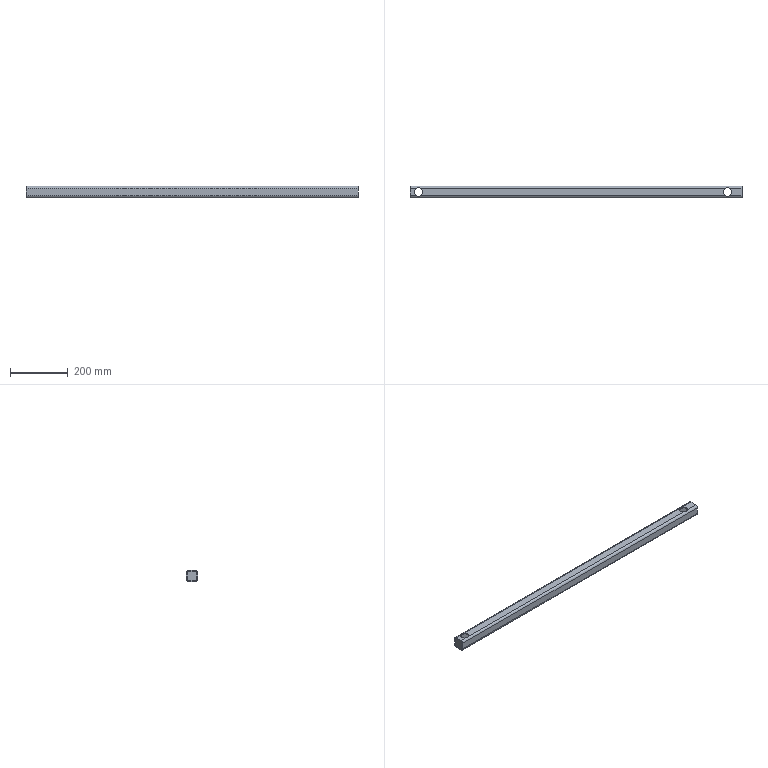Part | STEP file | FAN_FRAME_PROFILEV11_Default<Machined> | 3 solids | 58 faces | box 1150 x 40 x 40 mm | volume 613608 mm3 | plane 30 | cylinder 28 | commonest cylinder face diameters 8 x12 30 x8 5 x4 16 x4